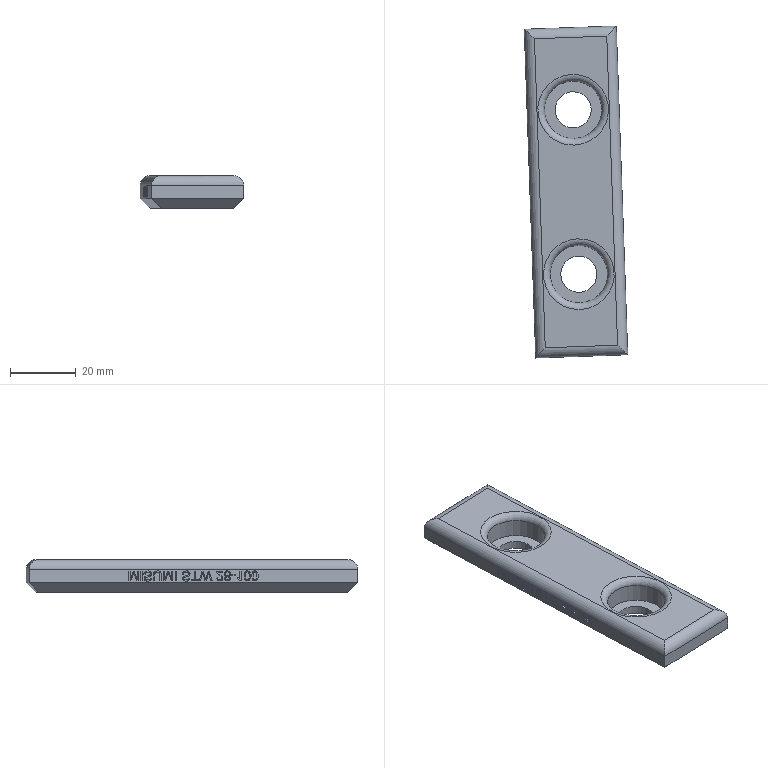Part | NX | features solid 2 | 1 solid | 146 faces | box 31.472 x 100.916 x 10 mm | volume 22209 mm3 | plane 96 | spline 40 | cylinder 8 | torus 2 | commonest cylinder face diameters 6 x4 11.007 x2 17.5 x2